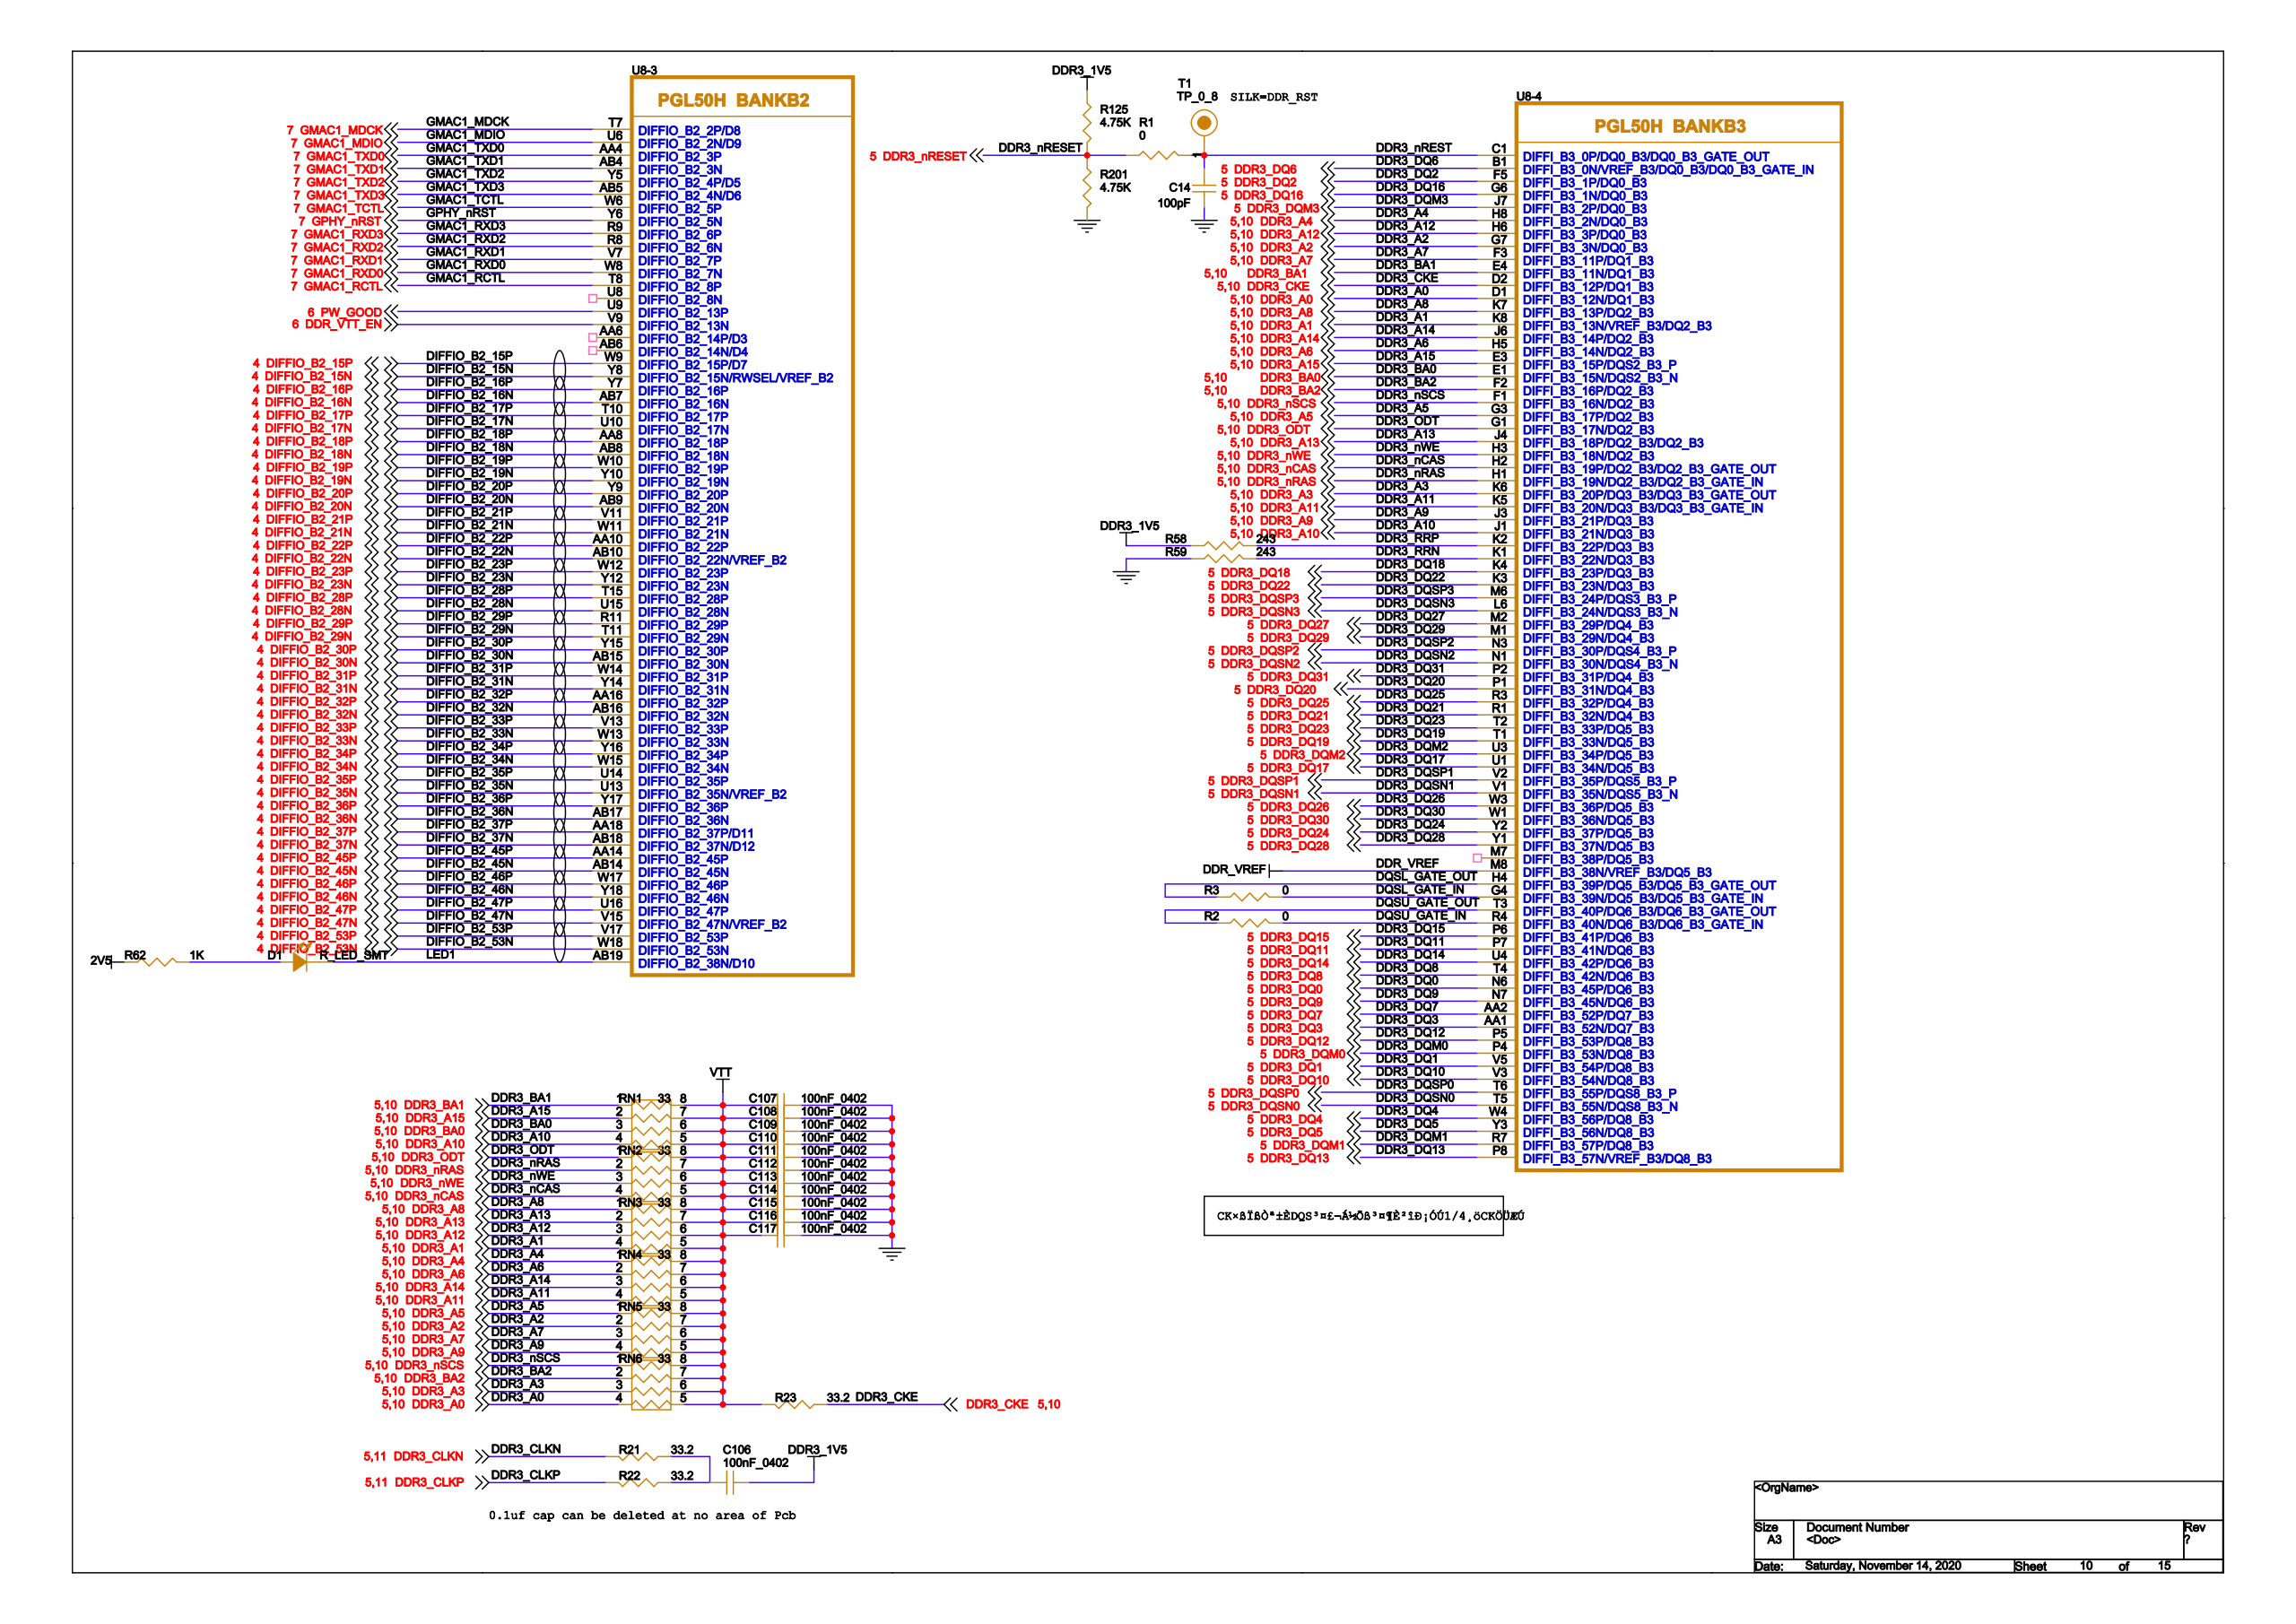Circuit board | Cadence Allegro | 406 parts | 392 nets | one sheet of the schematic
Parts on this sheet (reference | value | footprint):
C106 | 100nF_0402 | C_0402_BGA
C107 | 100nF_0402 | C_0402_BGA
C108 | 100nF_0402 | C_0402_BGA
C109 | 100nF_0402 | C_0402_BGA
C110 | 100nF_0402 | C_0402_BGA
C111 | 100nF_0402 | C_0402_BGA
C112 | 100nF_0402 | C_0402_BGA
C113 | 100nF_0402 | C_0402_BGA
C114 | 100nF_0402 | C_0402_BGA
C115 | 100nF_0402 | C_0402_BGA
C116 | 100nF_0402 | C_0402_BGA
C117 | 100nF_0402 | C_0402_BGA
D1 | R_LED_SMT | D_LED0805
R1 | 0 | R_0603
R2 | 0 | R_0603
R3 | 0 | R_0603
R21 | 33.2 | R_0603
R22 | 33.2 | R_0603
R23 | 33.2 | R_0603
R58 | 243 | R_0603
R59 | 243 | R_0603
R62 | 1K | R_0603
R125 | 4.75K | R_0603
R201 | 4.75K | R_0603
T1 | TP_0_8 | TP_0_8
U1 | RTL8211FI-CG | U_QFN40_0_4
U3 | RTL8201FI-VC-CG | U_QFN32_0_5
U4 | RTL8201FI-VC-CG | U_QFN32_0_5
U8 | PGL50H-7IFBGA484 | U_FBGA484_1_0
U16 | HXI15H4G160AF-13K | U_TFBGA96
Nets of these parts (net: part-pin ...):
GND: C107-2 C108-2 C109-2 C110-2 C111-2 C112-2 C113-2 C114-2 C115-2 C116-2 C117-2 R59-1 R201-1 U3-33 U4-33 U8-C14 U16-B1 U16-D1 U16-E1 U16-G1 U16-M1 U16-P1 U16-T1
DIFFIO_B2_35N: U8-U13
DIFFIO_B2_35P: U8-U14
DIFFIO_B2_45P: U8-AA14
DIFFIO_B2_45N: U8-AB14
DIFFIO_B2_47N: U8-V15
DIFFIO_B2_47P: U8-U16
DIFFIO_B2_46N: U8-Y18
DIFFIO_B2_46P: U8-W17
DIFFIO_B2_34N: U8-W15
DIFFIO_B2_34P: U8-Y16
DIFFIO_B2_33N: U8-W13
DIFFIO_B2_33P: U8-V13
DIFFIO_B2_53P: U8-V17
DIFFIO_B2_53N: U8-W18
DIFFIO_B2_32P: U8-AA16
DIFFIO_B2_32N: U8-AB16
DIFFIO_B2_31P: U8-W14
DIFFIO_B2_31N: U8-Y14
DIFFIO_B2_30P: U8-Y15
DIFFIO_B2_30N: U8-AB15
DIFFIO_B2_15P: U8-W9
DIFFIO_B2_15N: U8-Y8
DIFFIO_B2_18P: U8-AA8
DIFFIO_B2_18N: U8-AB8
DIFFIO_B2_17P: U8-T10
DIFFIO_B2_17N: U8-U10
DIFFIO_B2_20N: U8-AB9
DIFFIO_B2_20P: U8-Y9
DIFFIO_B2_21P: U8-V11
DIFFIO_B2_21N: U8-W11
DIFFIO_B2_22P: U8-AA10
DIFFIO_B2_22N: U8-AB10
DIFFIO_B2_16P: U8-Y7
DIFFIO_B2_16N: U8-AB7
DIFFIO_B2_19P: U8-W10
DIFFIO_B2_19N: U8-Y10
DIFFIO_B2_23P: U8-W12
DIFFIO_B2_23N: U8-Y12
DIFFIO_B2_28P: U8-T15
DIFFIO_B2_28N: U8-U15
DIFFIO_B2_29P: U8-R11
DIFFIO_B2_29N: U8-T11
DIFFIO_B2_36P: U8-Y17
DIFFIO_B2_36N: U8-AB17
DIFFIO_B2_37P: U8-AA18
DIFFIO_B2_37N: U8-AB18
N20056743: D1-1 R62-2
LED1: D1-2 U8-AB19
DDR3_1V5: C106-1 R58-1 R125-2 U8-R2 U16-C1 U16-D2 U16-F1 U16-G7 U16-H2 U16-K2 U16-K8 U16-N1 U16-R1 U16-R9
N20059952: C106-2 R21-1 R22-1
VTT: C107-1 C108-1 C109-1 C110-1 C111-1 C112-1 C113-1 C114-1 C115-1 C116-1 C117-1 R23-2
DDR_VREF: U8-M8 U16-H1 U16-M8
DDR3_NREST: R1-1 T1-1 U8-C1
DDR_VTT_EN: U8-V9
2V5: R62-1
DDR3_NRESET: R1-2 R125-1 R201-2 U16-T2
DQSU_GATE_OUT: R2-1 U8-T3
DQSU_GATE_IN: R2-2 U8-R4
DQSL_GATE_OUT: R3-1 U8-H4
DQSL_GATE_IN: R3-2 U8-G4
GMAC1_RXD3: U8-R9
GMAC1_RCTL: U8-T8
PW_GOOD: U8-U9
DDR3_CLKN: R21-2 U16-K7
DDR3_CLKP: R22-2 U16-J7
DDR3_CKE: R23-1 U8-D2
DDR3_RRP: R58-2 U8-K2
DDR3_RRN: R59-2 U8-K1
GMAC1_MDIO: U1-14 U8-U6
DDR3_BA1: U8-E4
DDR3_A15: U8-E3 U16-M7
DDR3_BA0: U8-E1 U16-M2
DDR3_A10: U8-J1
DDR3_ODT: U8-G1 U16-K1
DDR3_A8: U8-K7 U16-T8
DDR3_A13: U8-J4 U16-T3
DDR3_A12: U8-H6 U16-N7
DDR3_A1: U8-K8 U16-P7
DDR3_A4: U8-H8 U16-P8
DDR3_A6: U8-H5 U16-R8
DDR3_A14: U8-J6 U16-T7
DDR3_A11: U8-K5 U16-R7
DDR3_A5: U8-G3 U16-P2
DDR3_A2: U8-G7
DDR3_A7: U8-F3 U16-R2
DDR3_A9: U8-J3 U16-R3
DDR3_BA2: U8-F2
DDR3_A3: U8-K6
DDR3_A0: U8-D1 U16-N3
GMAC1_MDCK: U8-T7
GMAC1_RXD0: U8-W8
GMAC1_RXD1: U8-V7
GMAC1_RXD2: U8-R8
GMAC1_TCTL: U8-W6
GMAC1_TXD0: U8-AA4
GMAC1_TXD1: U8-AB4
GMAC1_TXD2: U8-Y5
GMAC1_TXD3: U1-15 U8-AB5
DDR3_DQM0: U8-P4
DDR3_DQM1: U8-R7
DDR3_DQ0: U8-N6 U16-E3
DDR3_DQ1: U8-V5
DDR3_DQ2: U8-F5 U16-F2
DDR3_DQ3: U8-AA1
DDR3_DQ4: U8-W4 U16-H3
DDR3_DQ5: U8-Y3 U16-H8
DDR3_DQ6: U8-B1
DDR3_DQ7: U8-AA2
DDR3_DQSP0: U8-T6 U16-F3
DDR3_DQSP1: U8-V2
DDR3_DQ8: U8-T4
DDR3_DQ9: U8-N7
DDR3_DQ10: U8-V3
DDR3_DQ11: U8-P7
DDR3_DQ12: U8-P5
DDR3_DQ13: U8-P8
DDR3_DQ14: U8-U4
DDR3_DQ15: U8-P6 U16-A3
DDR3_DQSN0: U8-T5 U16-G3
DDR3_DQSN1: U8-V1
DDR3_DQM2: U8-U3
DDR3_DQM3: U8-J7
DDR3_DQ16: U8-G6
DDR3_DQ17: U8-U1
DDR3_DQ18: U8-K4
DDR3_DQ19: U8-T1
DDR3_DQ20: U8-P1
DDR3_DQ21: U8-R1
DDR3_DQ22: U8-K3
DDR3_DQ23: U8-T2
DDR3_DQSP2: U8-N3
DDR3_DQSP3: U8-M6
DDR3_DQ24: U8-Y2
DDR3_DQ25: U8-R3
DDR3_DQ26: U8-W3
DDR3_DQ27: U8-M2
DDR3_DQ28: U8-Y1
DDR3_DQ29: U8-M1
DDR3_DQ30: U8-W1
DDR3_DQ31: U8-P2
DDR3_DQSN2: U8-N1
DDR3_DQSN3: U8-L6